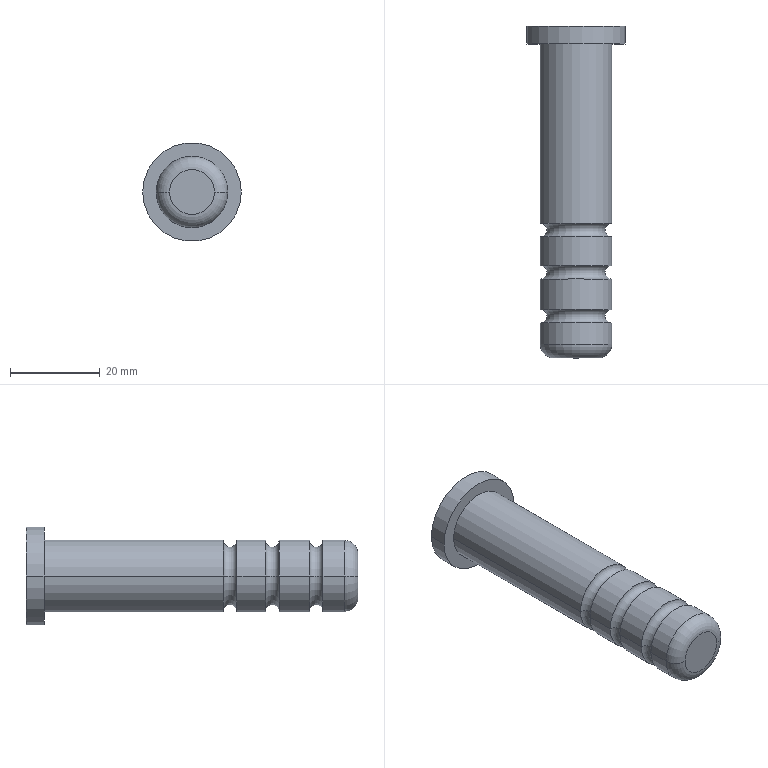Part | Creo | features DATUM PLANE 3, COORDINATE SYSTEM 1, CURVE 1, PROTRUSION 1 | 1 solid | 21 faces | box 22 x 74 x 22 mm | volume 15015 mm3 | cylinder 10 | torus 8 | plane 3 | commonest cylinder face diameters 16 x8 22 x2
STEP:
#1=CARTESIAN_POINT('',(0.,0.,0.));
#2=DIRECTION('',(0.,0.,1.));
#3=DIRECTION('',(1.,0.,0.));
#4=AXIS2_PLACEMENT_3D('',#1,#2,#3);
#5=CARTESIAN_POINT('',(8.,3.,0.));
#6=VERTEX_POINT('',#5);
#7=CARTESIAN_POINT('',(8.,7.793,0.));
#8=VERTEX_POINT('',#7);
#9=CARTESIAN_POINT('',(8.,3.,0.));
#10=DIRECTION('',(0.,1.,0.));
#11=VECTOR('',#10,4.793);
#12=LINE('',#9,#11);
#13=EDGE_CURVE('',#6,#8,#12,.T.);
#14=ORIENTED_EDGE('',*,*,#13,.T.);
#15=CARTESIAN_POINT('',(-8.,7.793,0.));
#16=VERTEX_POINT('',#15);
#17=CARTESIAN_POINT('',(0.,7.793,0.));
#18=DIRECTION('',(0.,1.,0.));
#19=DIRECTION('',(1.,0.,0.));
#20=AXIS2_PLACEMENT_3D('',#17,#18,#19);
#21=CIRCLE('',#20,8.);
#22=EDGE_CURVE('',#8,#16,#21,.T.);
#23=ORIENTED_EDGE('',*,*,#22,.T.);
#24=CARTESIAN_POINT('',(-8.,3.,0.));
#25=VERTEX_POINT('',#24);
#26=CARTESIAN_POINT('',(-8.,3.,0.));
#27=DIRECTION('',(0.,1.,0.));
#28=VECTOR('',#27,4.793);
#29=LINE('',#26,#28);
#30=EDGE_CURVE('',#25,#16,#29,.T.);
#31=ORIENTED_EDGE('',*,*,#30,.F.);
#32=CARTESIAN_POINT('',(0.,3.,0.));
#33=DIRECTION('',(0.,1.,0.));
#34=DIRECTION('',(1.,0.,0.));
#35=AXIS2_PLACEMENT_3D('',#32,#33,#34);
#36=CIRCLE('',#35,8.);
#37=EDGE_CURVE('',#6,#25,#36,.T.);
#38=ORIENTED_EDGE('',*,*,#37,.F.);
#39=EDGE_LOOP('',(#14,#23,#31,#38));
#40=FACE_OUTER_BOUND('',#39,.F.);
#41=CARTESIAN_POINT('',(0.,0.,0.));
#42=DIRECTION('',(0.,1.,0.));
#43=DIRECTION('',(1.,0.,0.));
#44=AXIS2_PLACEMENT_3D('',#41,#42,#43);
#45=CYLINDRICAL_SURFACE('',#44,8.);
#46=ADVANCED_FACE('',(#40),#45,.T.);
#47=ORIENTED_EDGE('',*,*,#13,.F.);
#48=CARTESIAN_POINT('',(0.,3.,0.));
#49=DIRECTION('',(0.,-1.,0.));
#50=DIRECTION('',(1.,0.,0.));
#51=AXIS2_PLACEMENT_3D('',#48,#49,#50);
#52=CIRCLE('',#51,8.);
#53=EDGE_CURVE('',#6,#25,#52,.T.);
#54=ORIENTED_EDGE('',*,*,#53,.T.);
#55=ORIENTED_EDGE('',*,*,#30,.T.);
#56=CARTESIAN_POINT('',(0.,7.793,0.));
#57=DIRECTION('',(0.,-1.,0.));
#58=DIRECTION('',(1.,0.,0.));
#59=AXIS2_PLACEMENT_3D('',#56,#57,#58);
#60=CIRCLE('',#59,8.);
#61=EDGE_CURVE('',#8,#16,#60,.T.);
#62=ORIENTED_EDGE('',*,*,#61,.F.);
#63=EDGE_LOOP('',(#47,#54,#55,#62));
#64=FACE_OUTER_BOUND('',#63,.F.);
#65=CARTESIAN_POINT('',(0.,0.,0.));
#66=DIRECTION('',(0.,1.,0.));
#67=DIRECTION('',(1.,0.,0.));
#68=AXIS2_PLACEMENT_3D('',#65,#66,#67);
#69=CYLINDRICAL_SURFACE('',#68,8.);
#70=ADVANCED_FACE('',(#64),#69,.T.);
#71=CARTESIAN_POINT('',(5.,0.,0.));
#72=VERTEX_POINT('',#71);
#73=CARTESIAN_POINT('',(5.,3.,0.));
#74=DIRECTION('',(0.,0.,1.));
#75=DIRECTION('',(0.,-1.,0.));
#76=AXIS2_PLACEMENT_3D('',#73,#74,#75);
#77=CIRCLE('',#76,3.);
#78=EDGE_CURVE('',#72,#6,#77,.T.);
#79=ORIENTED_EDGE('',*,*,#78,.F.);
#80=CARTESIAN_POINT('',(-5.,0.,0.));
#81=VERTEX_POINT('',#80);
#82=CARTESIAN_POINT('',(0.,0.,0.));
#83=DIRECTION('',(0.,-1.,0.));
#84=DIRECTION('',(1.,0.,0.));
#85=AXIS2_PLACEMENT_3D('',#82,#83,#84);
#86=CIRCLE('',#85,5.);
#87=EDGE_CURVE('',#72,#81,#86,.T.);
#88=ORIENTED_EDGE('',*,*,#87,.T.);
#89=CARTESIAN_POINT('',(-5.,3.,0.));
#90=DIRECTION('',(0.,0.,-1.));
#91=DIRECTION('',(0.,-1.,0.));
#92=AXIS2_PLACEMENT_3D('',#89,#90,#91);
#93=CIRCLE('',#92,3.);
#94=EDGE_CURVE('',#81,#25,#93,.T.);
#95=ORIENTED_EDGE('',*,*,#94,.T.);
#96=ORIENTED_EDGE('',*,*,#53,.F.);
#97=EDGE_LOOP('',(#79,#88,#95,#96));
#98=FACE_OUTER_BOUND('',#97,.F.);
#99=CARTESIAN_POINT('',(0.,3.,0.));
#100=DIRECTION('',(0.,1.,0.));
#101=DIRECTION('',(1.,0.,0.));
#102=AXIS2_PLACEMENT_3D('',#99,#100,#101);
#103=TOROIDAL_SURFACE('',#102,5.,3.);
#104=ADVANCED_FACE('',(#98),#103,.T.);
#105=ORIENTED_EDGE('',*,*,#78,.T.);
#106=ORIENTED_EDGE('',*,*,#37,.T.);
#107=ORIENTED_EDGE('',*,*,#94,.F.);
#108=CARTESIAN_POINT('',(0.,0.,0.));
#109=DIRECTION('',(0.,1.,0.));
#110=DIRECTION('',(1.,0.,0.));
#111=AXIS2_PLACEMENT_3D('',#108,#109,#110);
#112=CIRCLE('',#111,5.);
#113=EDGE_CURVE('',#72,#81,#112,.T.);
#114=ORIENTED_EDGE('',*,*,#113,.F.);
#115=EDGE_LOOP('',(#105,#106,#107,#114));
#116=FACE_OUTER_BOUND('',#115,.F.);
#117=CARTESIAN_POINT('',(0.,3.,0.));
#118=DIRECTION('',(0.,1.,0.));
#119=DIRECTION('',(1.,0.,0.));
#120=AXIS2_PLACEMENT_3D('',#117,#118,#119);
#121=TOROIDAL_SURFACE('',#120,5.,3.);
#122=ADVANCED_FACE('',(#116),#121,.T.);
#123=ORIENTED_EDGE('',*,*,#87,.F.);
#124=ORIENTED_EDGE('',*,*,#113,.T.);
#125=EDGE_LOOP('',(#123,#124));
#126=FACE_OUTER_BOUND('',#125,.F.);
#127=CARTESIAN_POINT('',(0.,0.,0.));
#128=DIRECTION('',(0.,1.,0.));
#129=DIRECTION('',(1.,0.,0.));
#130=AXIS2_PLACEMENT_3D('',#127,#128,#129);
#131=PLANE('',#130);
#132=ADVANCED_FACE('',(#126),#131,.F.);
#133=CARTESIAN_POINT('',(8.,10.793,0.));
#134=VERTEX_POINT('',#133);
#135=CARTESIAN_POINT('',(8.,9.293,0.));
#136=DIRECTION('',(0.,0.,-1.));
#137=DIRECTION('',(0.,-1.,0.));
#138=AXIS2_PLACEMENT_3D('',#135,#136,#137);
#139=CIRCLE('',#138,1.5);
#140=EDGE_CURVE('',#8,#134,#139,.T.);
#141=ORIENTED_EDGE('',*,*,#140,.F.);
#142=ORIENTED_EDGE('',*,*,#61,.T.);
#143=CARTESIAN_POINT('',(-8.,10.793,0.));
#144=VERTEX_POINT('',#143);
#145=CARTESIAN_POINT('',(-8.,9.293,0.));
#146=DIRECTION('',(0.,0.,1.));
#147=DIRECTION('',(0.,-1.,0.));
#148=AXIS2_PLACEMENT_3D('',#145,#146,#147);
#149=CIRCLE('',#148,1.5);
#150=EDGE_CURVE('',#16,#144,#149,.T.);
#151=ORIENTED_EDGE('',*,*,#150,.T.);
#152=CARTESIAN_POINT('',(0.,10.793,0.));
#153=DIRECTION('',(0.,-1.,0.));
#154=DIRECTION('',(1.,0.,0.));
#155=AXIS2_PLACEMENT_3D('',#152,#153,#154);
#156=CIRCLE('',#155,8.);
#157=EDGE_CURVE('',#134,#144,#156,.T.);
#158=ORIENTED_EDGE('',*,*,#157,.F.);
#159=EDGE_LOOP('',(#141,#142,#151,#158));
#160=FACE_OUTER_BOUND('',#159,.F.);
#161=CARTESIAN_POINT('',(0.,9.293,0.));
#162=DIRECTION('',(0.,1.,0.));
#163=DIRECTION('',(1.,0.,0.));
#164=AXIS2_PLACEMENT_3D('',#161,#162,#163);
#165=TOROIDAL_SURFACE('',#164,8.,1.5);
#166=ADVANCED_FACE('',(#160),#165,.F.);
#167=ORIENTED_EDGE('',*,*,#140,.T.);
#168=CARTESIAN_POINT('',(0.,10.793,0.));
#169=DIRECTION('',(0.,1.,0.));
#170=DIRECTION('',(1.,0.,0.));
#171=AXIS2_PLACEMENT_3D('',#168,#169,#170);
#172=CIRCLE('',#171,8.);
#173=EDGE_CURVE('',#134,#144,#172,.T.);
#174=ORIENTED_EDGE('',*,*,#173,.T.);
#175=ORIENTED_EDGE('',*,*,#150,.F.);
#176=ORIENTED_EDGE('',*,*,#22,.F.);
#177=EDGE_LOOP('',(#167,#174,#175,#176));
#178=FACE_OUTER_BOUND('',#177,.F.);
#179=CARTESIAN_POINT('',(0.,9.293,0.));
#180=DIRECTION('',(0.,1.,0.));
#181=DIRECTION('',(1.,0.,0.));
#182=AXIS2_PLACEMENT_3D('',#179,#180,#181);
#183=TOROIDAL_SURFACE('',#182,8.,1.5);
#184=ADVANCED_FACE('',(#178),#183,.F.);
#185=CARTESIAN_POINT('',(8.,17.593,0.));
#186=VERTEX_POINT('',#185);
#187=CARTESIAN_POINT('',(8.,10.793,0.));
#188=DIRECTION('',(0.,1.,0.));
#189=VECTOR('',#188,6.8);
#190=LINE('',#187,#189);
#191=EDGE_CURVE('',#134,#186,#190,.T.);
#192=ORIENTED_EDGE('',*,*,#191,.T.);
#193=CARTESIAN_POINT('',(-8.,17.593,0.));
#194=VERTEX_POINT('',#193);
#195=CARTESIAN_POINT('',(0.,17.593,0.));
#196=DIRECTION('',(0.,1.,0.));
#197=DIRECTION('',(1.,0.,0.));
#198=AXIS2_PLACEMENT_3D('',#195,#196,#197);
#199=CIRCLE('',#198,8.);
#200=EDGE_CURVE('',#186,#194,#199,.T.);
#201=ORIENTED_EDGE('',*,*,#200,.T.);
#202=CARTESIAN_POINT('',(-8.,10.793,0.));
#203=DIRECTION('',(0.,1.,0.));
#204=VECTOR('',#203,6.8);
#205=LINE('',#202,#204);
#206=EDGE_CURVE('',#144,#194,#205,.T.);
#207=ORIENTED_EDGE('',*,*,#206,.F.);
#208=ORIENTED_EDGE('',*,*,#173,.F.);
#209=EDGE_LOOP('',(#192,#201,#207,#208));
#210=FACE_OUTER_BOUND('',#209,.F.);
#211=CARTESIAN_POINT('',(0.,0.,0.));
#212=DIRECTION('',(0.,1.,0.));
#213=DIRECTION('',(1.,0.,0.));
#214=AXIS2_PLACEMENT_3D('',#211,#212,#213);
#215=CYLINDRICAL_SURFACE('',#214,8.);
#216=ADVANCED_FACE('',(#210),#215,.T.);
#217=ORIENTED_EDGE('',*,*,#191,.F.);
#218=ORIENTED_EDGE('',*,*,#157,.T.);
#219=ORIENTED_EDGE('',*,*,#206,.T.);
#220=CARTESIAN_POINT('',(0.,17.593,0.));
#221=DIRECTION('',(0.,-1.,0.));
#222=DIRECTION('',(1.,0.,0.));
#223=AXIS2_PLACEMENT_3D('',#220,#221,#222);
#224=CIRCLE('',#223,8.);
#225=EDGE_CURVE('',#186,#194,#224,.T.);
#226=ORIENTED_EDGE('',*,*,#225,.F.);
#227=EDGE_LOOP('',(#217,#218,#219,#226));
#228=FACE_OUTER_BOUND('',#227,.F.);
#229=CARTESIAN_POINT('',(0.,0.,0.));
#230=DIRECTION('',(0.,1.,0.));
#231=DIRECTION('',(1.,0.,0.));
#232=AXIS2_PLACEMENT_3D('',#229,#230,#231);
#233=CYLINDRICAL_SURFACE('',#232,8.);
#234=ADVANCED_FACE('',(#228),#233,.T.);
#235=CARTESIAN_POINT('',(8.,20.593,0.));
#236=VERTEX_POINT('',#235);
#237=CARTESIAN_POINT('',(8.,19.093,0.));
#238=DIRECTION('',(0.,0.,-1.));
#239=DIRECTION('',(0.,-1.,0.));
#240=AXIS2_PLACEMENT_3D('',#237,#238,#239);
#241=CIRCLE('',#240,1.5);
#242=EDGE_CURVE('',#186,#236,#241,.T.);
#243=ORIENTED_EDGE('',*,*,#242,.F.);
#244=ORIENTED_EDGE('',*,*,#225,.T.);
#245=CARTESIAN_POINT('',(-8.,20.593,0.));
#246=VERTEX_POINT('',#245);
#247=CARTESIAN_POINT('',(-8.,19.093,0.));
#248=DIRECTION('',(0.,0.,1.));
#249=DIRECTION('',(0.,-1.,0.));
#250=AXIS2_PLACEMENT_3D('',#247,#248,#249);
#251=CIRCLE('',#250,1.5);
#252=EDGE_CURVE('',#194,#246,#251,.T.);
#253=ORIENTED_EDGE('',*,*,#252,.T.);
#254=CARTESIAN_POINT('',(0.,20.593,0.));
#255=DIRECTION('',(0.,-1.,0.));
#256=DIRECTION('',(1.,0.,0.));
#257=AXIS2_PLACEMENT_3D('',#254,#255,#256);
#258=CIRCLE('',#257,8.);
#259=EDGE_CURVE('',#236,#246,#258,.T.);
#260=ORIENTED_EDGE('',*,*,#259,.F.);
#261=EDGE_LOOP('',(#243,#244,#253,#260));
#262=FACE_OUTER_BOUND('',#261,.F.);
#263=CARTESIAN_POINT('',(0.,19.093,0.));
#264=DIRECTION('',(0.,1.,0.));
#265=DIRECTION('',(1.,0.,0.));
#266=AXIS2_PLACEMENT_3D('',#263,#264,#265);
#267=TOROIDAL_SURFACE('',#266,8.,1.5);
#268=ADVANCED_FACE('',(#262),#267,.F.);
#269=ORIENTED_EDGE('',*,*,#242,.T.);
#270=CARTESIAN_POINT('',(0.,20.593,0.));
#271=DIRECTION('',(0.,1.,0.));
#272=DIRECTION('',(1.,0.,0.));
#273=AXIS2_PLACEMENT_3D('',#270,#271,#272);
#274=CIRCLE('',#273,8.);
#275=EDGE_CURVE('',#236,#246,#274,.T.);
#276=ORIENTED_EDGE('',*,*,#275,.T.);
#277=ORIENTED_EDGE('',*,*,#252,.F.);
#278=ORIENTED_EDGE('',*,*,#200,.F.);
#279=EDGE_LOOP('',(#269,#276,#277,#278));
#280=FACE_OUTER_BOUND('',#279,.F.);
#281=CARTESIAN_POINT('',(0.,19.093,0.));
#282=DIRECTION('',(0.,1.,0.));
#283=DIRECTION('',(1.,0.,0.));
#284=AXIS2_PLACEMENT_3D('',#281,#282,#283);
#285=TOROIDAL_SURFACE('',#284,8.,1.5);
#286=ADVANCED_FACE('',(#280),#285,.F.);
#287=CARTESIAN_POINT('',(8.,27.,0.));
#288=VERTEX_POINT('',#287);
#289=CARTESIAN_POINT('',(8.,20.593,0.));
#290=DIRECTION('',(0.,1.,0.));
#291=VECTOR('',#290,6.407);
#292=LINE('',#289,#291);
#293=EDGE_CURVE('',#236,#288,#292,.T.);
#294=ORIENTED_EDGE('',*,*,#293,.T.);
#295=CARTESIAN_POINT('',(-8.,27.,0.));
#296=VERTEX_POINT('',#295);
#297=CARTESIAN_POINT('',(0.,27.,0.));
#298=DIRECTION('',(0.,1.,0.));
#299=DIRECTION('',(1.,0.,0.));
#300=AXIS2_PLACEMENT_3D('',#297,#298,#299);
#301=CIRCLE('',#300,8.);
#302=EDGE_CURVE('',#288,#296,#301,.T.);
#303=ORIENTED_EDGE('',*,*,#302,.T.);
#304=CARTESIAN_POINT('',(-8.,20.593,0.));
#305=DIRECTION('',(0.,1.,0.));
#306=VECTOR('',#305,6.407);
#307=LINE('',#304,#306);
#308=EDGE_CURVE('',#246,#296,#307,.T.);
#309=ORIENTED_EDGE('',*,*,#308,.F.);
#310=ORIENTED_EDGE('',*,*,#275,.F.);
#311=EDGE_LOOP('',(#294,#303,#309,#310));
#312=FACE_OUTER_BOUND('',#311,.F.);
#313=CARTESIAN_POINT('',(0.,0.,0.));
#314=DIRECTION('',(0.,1.,0.));
#315=DIRECTION('',(1.,0.,0.));
#316=AXIS2_PLACEMENT_3D('',#313,#314,#315);
#317=CYLINDRICAL_SURFACE('',#316,8.);
#318=ADVANCED_FACE('',(#312),#317,.T.);
#319=ORIENTED_EDGE('',*,*,#293,.F.);
#320=ORIENTED_EDGE('',*,*,#259,.T.);
#321=ORIENTED_EDGE('',*,*,#308,.T.);
#322=CARTESIAN_POINT('',(0.,27.,0.));
#323=DIRECTION('',(0.,-1.,0.));
#324=DIRECTION('',(1.,0.,0.));
#325=AXIS2_PLACEMENT_3D('',#322,#323,#324);
#326=CIRCLE('',#325,8.);
#327=EDGE_CURVE('',#288,#296,#326,.T.);
#328=ORIENTED_EDGE('',*,*,#327,.F.);
#329=EDGE_LOOP('',(#319,#320,#321,#328));
#330=FACE_OUTER_BOUND('',#329,.F.);
#331=CARTESIAN_POINT('',(0.,0.,0.));
#332=DIRECTION('',(0.,1.,0.));
#333=DIRECTION('',(1.,0.,0.));
#334=AXIS2_PLACEMENT_3D('',#331,#332,#333);
#335=CYLINDRICAL_SURFACE('',#334,8.);
#336=ADVANCED_FACE('',(#330),#335,.T.);
#337=CARTESIAN_POINT('',(8.,30.,0.));
#338=VERTEX_POINT('',#337);
#339=CARTESIAN_POINT('',(8.,28.5,0.));
#340=DIRECTION('',(0.,0.,-1.));
#341=DIRECTION('',(0.,-1.,0.));
#342=AXIS2_PLACEMENT_3D('',#339,#340,#341);
#343=CIRCLE('',#342,1.5);
#344=EDGE_CURVE('',#288,#338,#343,.T.);
#345=ORIENTED_EDGE('',*,*,#344,.F.);
#346=ORIENTED_EDGE('',*,*,#327,.T.);
#347=CARTESIAN_POINT('',(-8.,30.,0.));
#348=VERTEX_POINT('',#347);
#349=CARTESIAN_POINT('',(-8.,28.5,0.));
#350=DIRECTION('',(0.,0.,1.));
#351=DIRECTION('',(0.,-1.,0.));
#352=AXIS2_PLACEMENT_3D('',#349,#350,#351);
#353=CIRCLE('',#352,1.5);
#354=EDGE_CURVE('',#296,#348,#353,.T.);
#355=ORIENTED_EDGE('',*,*,#354,.T.);
#356=CARTESIAN_POINT('',(0.,30.,0.));
#357=DIRECTION('',(0.,-1.,0.));
#358=DIRECTION('',(1.,0.,0.));
#359=AXIS2_PLACEMENT_3D('',#356,#357,#358);
#360=CIRCLE('',#359,8.);
#361=EDGE_CURVE('',#338,#348,#360,.T.);
#362=ORIENTED_EDGE('',*,*,#361,.F.);
#363=EDGE_LOOP('',(#345,#346,#355,#362));
#364=FACE_OUTER_BOUND('',#363,.F.);
#365=CARTESIAN_POINT('',(0.,28.5,0.));
#366=DIRECTION('',(0.,1.,0.));
#367=DIRECTION('',(1.,0.,0.));
#368=AXIS2_PLACEMENT_3D('',#365,#366,#367);
#369=TOROIDAL_SURFACE('',#368,8.,1.5);
#370=ADVANCED_FACE('',(#364),#369,.F.);
#371=ORIENTED_EDGE('',*,*,#344,.T.);
#372=CARTESIAN_POINT('',(0.,30.,0.));
#373=DIRECTION('',(0.,1.,0.));
#374=DIRECTION('',(1.,0.,0.));
#375=AXIS2_PLACEMENT_3D('',#372,#373,#374);
#376=CIRCLE('',#375,8.);
#377=EDGE_CURVE('',#338,#348,#376,.T.);
#378=ORIENTED_EDGE('',*,*,#377,.T.);
#379=ORIENTED_EDGE('',*,*,#354,.F.);
#380=ORIENTED_EDGE('',*,*,#302,.F.);
#381=EDGE_LOOP('',(#371,#378,#379,#380));
#382=FACE_OUTER_BOUND('',#381,.F.);
#383=CARTESIAN_POINT('',(0.,28.5,0.));
#384=DIRECTION('',(0.,1.,0.));
#385=DIRECTION('',(1.,0.,0.));
#386=AXIS2_PLACEMENT_3D('',#383,#384,#385);
#387=TOROIDAL_SURFACE('',#386,8.,1.5);
#388=ADVANCED_FACE('',(#382),#387,.F.);
#389=CARTESIAN_POINT('',(8.,70.,0.));
#390=VERTEX_POINT('',#389);
#391=CARTESIAN_POINT('',(8.,30.,0.));
#392=DIRECTION('',(0.,1.,0.));
#393=VECTOR('',#392,40.);
#394=LINE('',#391,#393);
#395=EDGE_CURVE('',#338,#390,#394,.T.);
#396=ORIENTED_EDGE('',*,*,#395,.T.);
#397=CARTESIAN_POINT('',(-8.,70.,0.));
#398=VERTEX_POINT('',#397);
#399=CARTESIAN_POINT('',(0.,70.,0.));
#400=DIRECTION('',(0.,1.,0.));
#401=DIRECTION('',(1.,0.,0.));
#402=AXIS2_PLACEMENT_3D('',#399,#400,#401);
#403=CIRCLE('',#402,8.);
#404=EDGE_CURVE('',#390,#398,#403,.T.);
#405=ORIENTED_EDGE('',*,*,#404,.T.);
#406=CARTESIAN_POINT('',(-8.,30.,0.));
#407=DIRECTION('',(0.,1.,0.));
#408=VECTOR('',#407,40.);
#409=LINE('',#406,#408);
#410=EDGE_CURVE('',#348,#398,#409,.T.);
#411=ORIENTED_EDGE('',*,*,#410,.F.);
#412=ORIENTED_EDGE('',*,*,#377,.F.);
#413=EDGE_LOOP('',(#396,#405,#411,#412));
#414=FACE_OUTER_BOUND('',#413,.F.);
#415=CARTESIAN_POINT('',(0.,0.,0.));
#416=DIRECTION('',(0.,1.,0.));
#417=DIRECTION('',(1.,0.,0.));
#418=AXIS2_PLACEMENT_3D('',#415,#416,#417);
#419=CYLINDRICAL_SURFACE('',#418,8.);
#420=ADVANCED_FACE('',(#414),#419,.T.);
#421=ORIENTED_EDGE('',*,*,#395,.F.);
#422=ORIENTED_EDGE('',*,*,#361,.T.);
#423=ORIENTED_EDGE('',*,*,#410,.T.);
#424=CARTESIAN_POINT('',(0.,70.,0.));
#425=DIRECTION('',(0.,-1.,0.));
#426=DIRECTION('',(1.,0.,0.));
#427=AXIS2_PLACEMENT_3D('',#424,#425,#426);
#428=CIRCLE('',#427,8.);
#429=EDGE_CURVE('',#390,#398,#428,.T.);
#430=ORIENTED_EDGE('',*,*,#429,.F.);
#431=EDGE_LOOP('',(#421,#422,#423,#430));
#432=FACE_OUTER_BOUND('',#431,.F.);
#433=CARTESIAN_POINT('',(0.,0.,0.));
#434=DIRECTION('',(0.,1.,0.));
#435=DIRECTION('',(1.,0.,0.));
#436=AXIS2_PLACEMENT_3D('',#433,#434,#435);
#437=CYLINDRICAL_SURFACE('',#436,8.);
#438=ADVANCED_FACE('',(#432),#437,.T.);
#439=CARTESIAN_POINT('',(11.,70.,0.));
#440=VERTEX_POINT('',#439);
#441=CARTESIAN_POINT('',(-11.,70.,0.));
#442=VERTEX_POINT('',#441);
#443=CARTESIAN_POINT('',(0.,70.,0.));
#444=DIRECTION('',(0.,1.,0.));
#445=DIRECTION('',(1.,0.,0.));
#446=AXIS2_PLACEMENT_3D('',#443,#444,#445);
#447=CIRCLE('',#446,11.);
#448=EDGE_CURVE('',#440,#442,#447,.T.);
#449=ORIENTED_EDGE('',*,*,#448,.T.);
#450=CARTESIAN_POINT('',(0.,70.,0.));
#451=DIRECTION('',(0.,-1.,0.));
#452=DIRECTION('',(1.,0.,0.));
#453=AXIS2_PLACEMENT_3D('',#450,#451,#452);
#454=CIRCLE('',#453,11.);
#455=EDGE_CURVE('',#440,#442,#454,.T.);
#456=ORIENTED_EDGE('',*,*,#455,.F.);
#457=EDGE_LOOP('',(#449,#456));
#458=FACE_OUTER_BOUND('',#457,.F.);
#459=ORIENTED_EDGE('',*,*,#429,.T.);
#460=ORIENTED_EDGE('',*,*,#404,.F.);
#461=EDGE_LOOP('',(#459,#460));
#462=FACE_BOUND('',#461,.F.);
#463=CARTESIAN_POINT('',(0.,70.,0.));
#464=DIRECTION('',(0.,1.,0.));
#465=DIRECTION('',(1.,0.,0.));
#466=AXIS2_PLACEMENT_3D('',#463,#464,#465);
#467=PLANE('',#466);
#468=ADVANCED_FACE('',(#458,#462),#467,.F.);
#469=CARTESIAN_POINT('',(11.,74.,0.));
#470=VERTEX_POINT('',#469);
#471=CARTESIAN_POINT('',(11.,70.,0.));
#472=DIRECTION('',(0.,1.,0.));
#473=VECTOR('',#472,4.);
#474=LINE('',#471,#473);
#475=EDGE_CURVE('',#440,#470,#474,.T.);
#476=ORIENTED_EDGE('',*,*,#475,.T.);
#477=CARTESIAN_POINT('',(-11.,74.,0.));
#478=VERTEX_POINT('',#477);
#479=CARTESIAN_POINT('',(0.,74.,0.));
#480=DIRECTION('',(0.,1.,0.));
#481=DIRECTION('',(1.,0.,0.));
#482=AXIS2_PLACEMENT_3D('',#479,#480,#481);
#483=CIRCLE('',#482,11.);
#484=EDGE_CURVE('',#470,#478,#483,.T.);
#485=ORIENTED_EDGE('',*,*,#484,.T.);
#486=CARTESIAN_POINT('',(-11.,70.,0.));
#487=DIRECTION('',(0.,1.,0.));
#488=VECTOR('',#487,4.);
#489=LINE('',#486,#488);
#490=EDGE_CURVE('',#442,#478,#489,.T.);
#491=ORIENTED_EDGE('',*,*,#490,.F.);
#492=ORIENTED_EDGE('',*,*,#448,.F.);
#493=EDGE_LOOP('',(#476,#485,#491,#492));
#494=FACE_OUTER_BOUND('',#493,.F.);
#495=CARTESIAN_POINT('',(0.,0.,0.));
#496=DIRECTION('',(0.,1.,0.));
#497=DIRECTION('',(1.,0.,0.));
#498=AXIS2_PLACEMENT_3D('',#495,#496,#497);
#499=CYLINDRICAL_SURFACE('',#498,11.);
#500=ADVANCED_FACE('',(#494),#499,.T.);
#501=ORIENTED_EDGE('',*,*,#475,.F.);
#502=ORIENTED_EDGE('',*,*,#455,.T.);
#503=ORIENTED_EDGE('',*,*,#490,.T.);
#504=CARTESIAN_POINT('',(0.,74.,0.));
#505=DIRECTION('',(0.,-1.,0.));
#506=DIRECTION('',(1.,0.,0.));
#507=AXIS2_PLACEMENT_3D('',#504,#505,#506);
#508=CIRCLE('',#507,11.);
#509=EDGE_CURVE('',#470,#478,#508,.T.);
#510=ORIENTED_EDGE('',*,*,#509,.F.);
#511=EDGE_LOOP('',(#501,#502,#503,#510));
#512=FACE_OUTER_BOUND('',#511,.F.);
#513=CARTESIAN_POINT('',(0.,0.,0.));
#514=DIRECTION('',(0.,1.,0.));
#515=DIRECTION('',(1.,0.,0.));
#516=AXIS2_PLACEMENT_3D('',#513,#514,#515);
#517=CYLINDRICAL_SURFACE('',#516,11.);
#518=ADVANCED_FACE('',(#512),#517,.T.);
#519=ORIENTED_EDGE('',*,*,#509,.T.);
#520=ORIENTED_EDGE('',*,*,#484,.F.);
#521=EDGE_LOOP('',(#519,#520));
#522=FACE_OUTER_BOUND('',#521,.F.);
#523=CARTESIAN_POINT('',(0.,74.,0.));
#524=DIRECTION('',(0.,1.,0.));
#525=DIRECTION('',(1.,0.,0.));
#526=AXIS2_PLACEMENT_3D('',#523,#524,#525);
#527=PLANE('',#526);
#528=ADVANCED_FACE('',(#522),#527,.T.);
#529=CLOSED_SHELL('',(#46,#70,#104,#122,#132,#166,#184,#216,#234,#268,#286,#318,#336,#370,#388,#420,#438,#468,#500,#518,#528));
#530=MANIFOLD_SOLID_BREP('',#529);
#531=(LENGTH_UNIT()NAMED_UNIT(*)SI_UNIT(.MILLI.,.METRE.));
#532=UNCERTAINTY_MEASURE_WITH_UNIT(LENGTH_MEASURE(0.008028),#531,'','');
#533=(NAMED_UNIT(*)PLANE_ANGLE_UNIT()SI_UNIT($,.RADIAN.));
#534=PLANE_ANGLE_MEASURE_WITH_UNIT(PLANE_ANGLE_MEASURE(0.01745),#533);
#535=(CONVERSION_BASED_UNIT('DEGREE',#534)NAMED_UNIT(*)PLANE_ANGLE_UNIT());
#536=(NAMED_UNIT(*)SI_UNIT($,.STERADIAN.)SOLID_ANGLE_UNIT());
#537=(GEOMETRIC_REPRESENTATION_CONTEXT(3)GLOBAL_UNCERTAINTY_ASSIGNED_CONTEXT((#532))GLOBAL_UNIT_ASSIGNED_CONTEXT((#531,#535,#536))REPRESENTATION_CONTEXT('',''));
#538=ADVANCED_BREP_SHAPE_REPRESENTATION('',(#4,#530),#537);